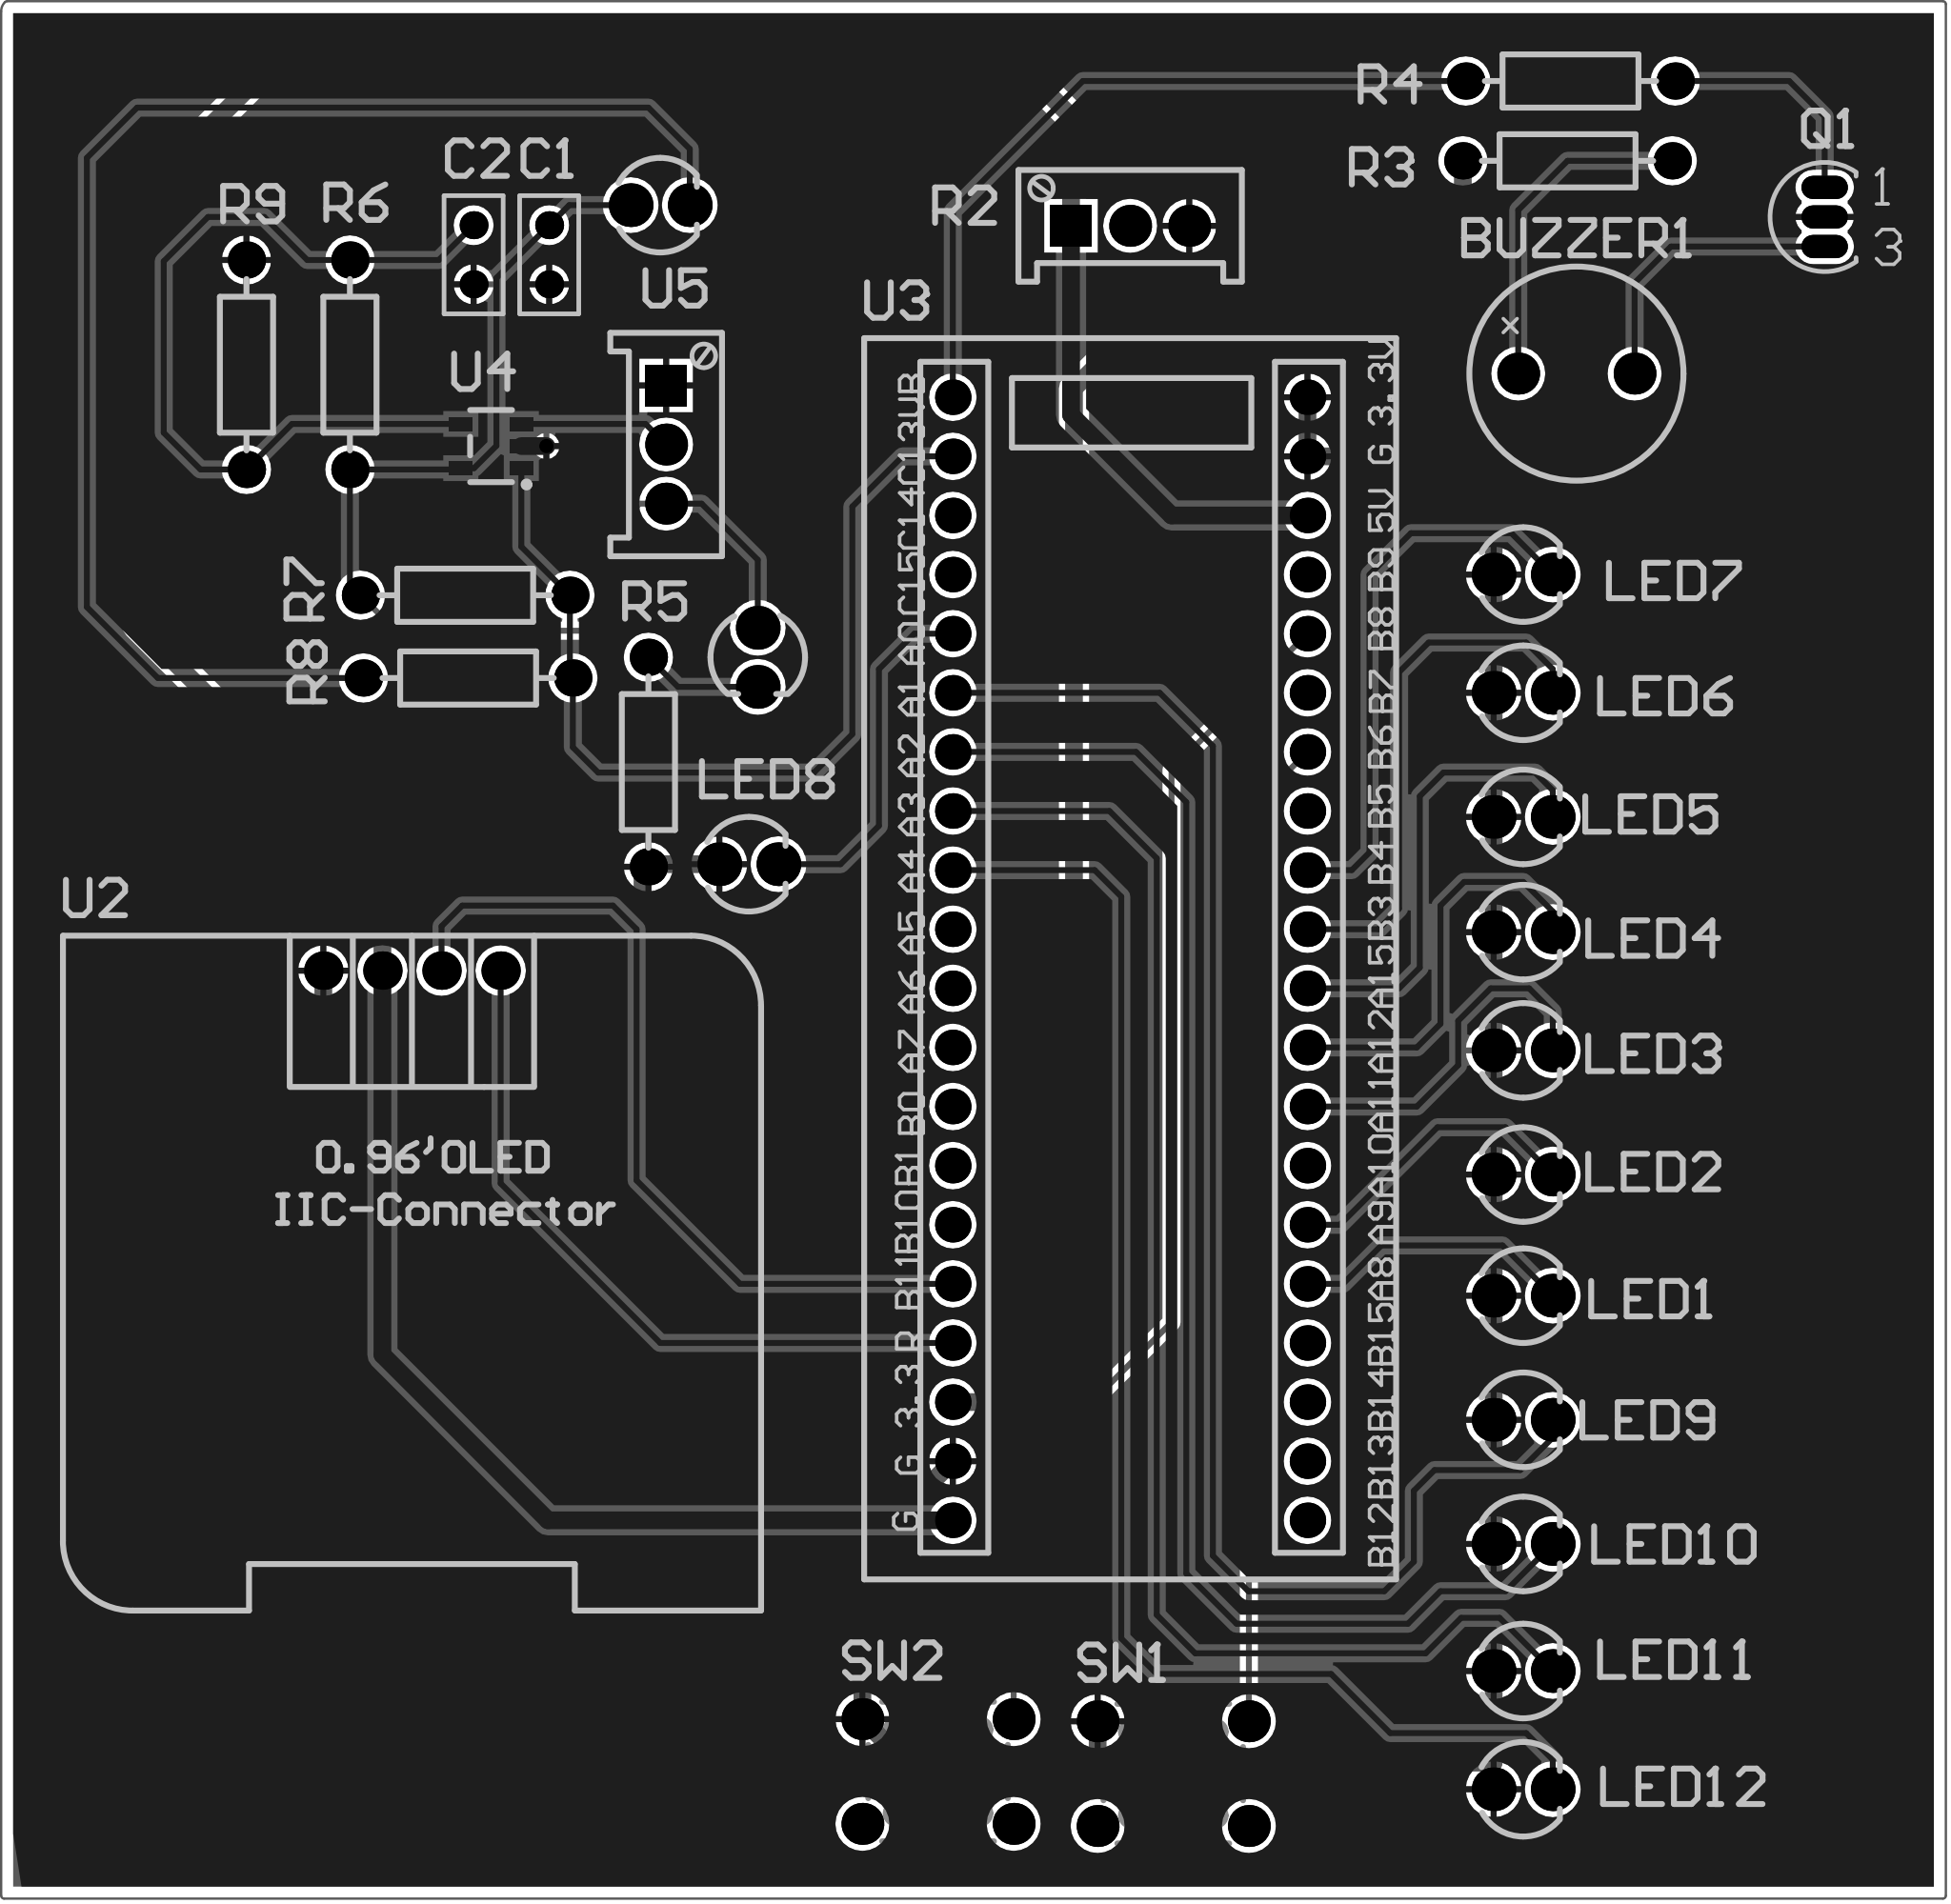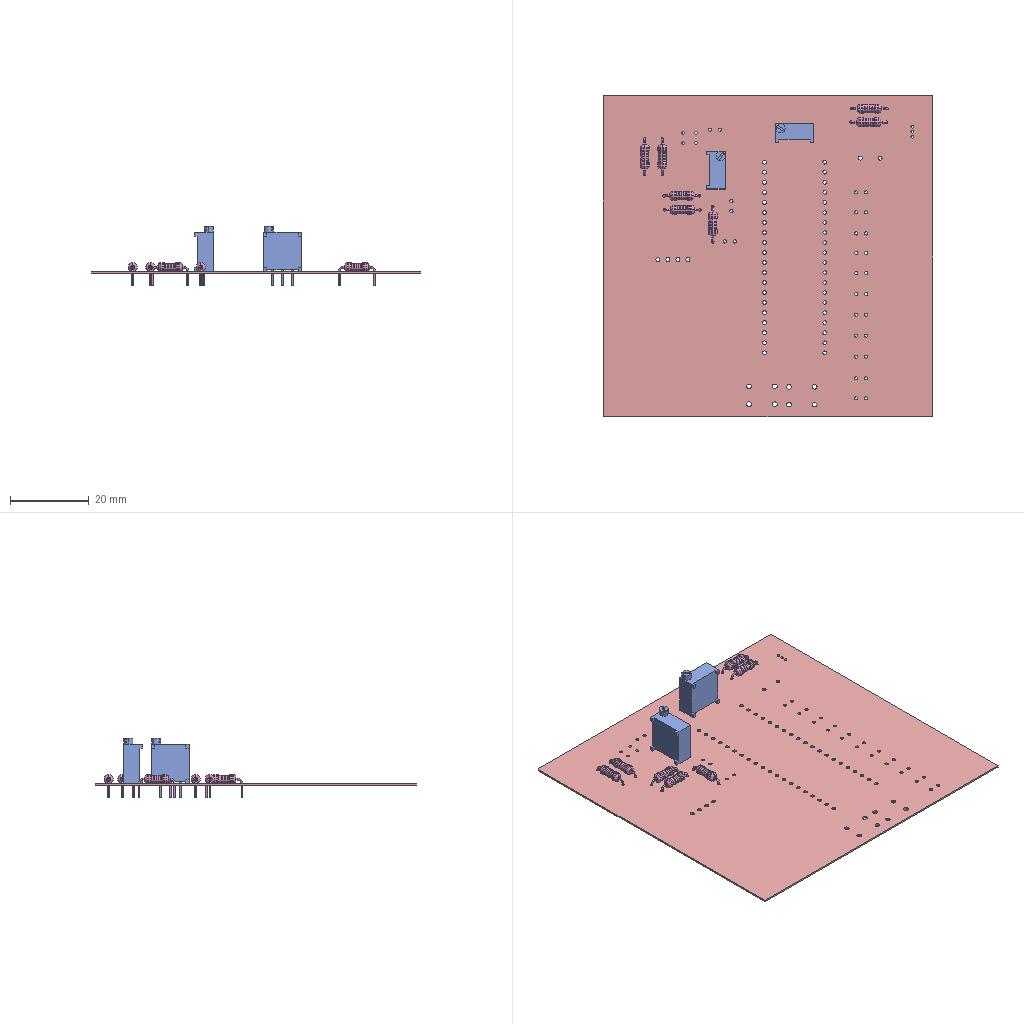Circuit board layout | Altium Designer | box 83.6 x 81.5 x 15 mm
Layer stack:
# Altium Designer layer stack of  (unit mm; dielectric type: 0 none, 1 core, 2 prepreg, 3 surface material)
index,name,kind,layer,copper_thickness_mm,dielectric_type,dielectric_thickness_mm,dielectric_material,dielectric_constant
0,Top Paste,other,,,,,,
1,Top Overlay,other,,,,,,
2,Top Solder,dielectric,,,3,0.0102,Solder Resist,3.5
3,Top Layer,copper,Top Layer,0.0356,,,,
4,Dielectric 1,dielectric,,,0,0.32,FR-4,4.8
5,Bottom Layer,copper,Bottom Layer,0.0356,,,,
6,Bottom Solder,dielectric,,,3,0.0102,Solder Resist,3.5
7,Bottom Overlay,other,,,,,,
8,Bottom Paste,other,,,,,,
# drill layer pairs: low layer,high layer
drill_pair,Top Layer,Bottom Layer
Part placement:
Designator,Comment,Layer,Footprint,Center-X(mm),Center-Y(mm),Rotation
电源指示,KT-0805G,TopLayer,LED3MM,98.933,87.503,270
开关指示,KT-0805G,TopLayer,LED3MM,94.742,106.934,360
U5,res2k3*3*1MM,TopLayer,3296W,94.996,96.647,270
U4,TLV3201AIDBVR,TopLayer,SOT-23-5_L3.0-W1.7-P0.95-LS2.8-BR,87.473,96.581,0
U3,LCKFB-DKX-STM32F103C8T6,TopLayer,STM32核心板,114.935,74.549,0
U2,HS96L03W2C03,TopLayer,0.96OLED_4P,84.074,74.04,0
SW2,TS-1101-C-W,TopLayer,四脚轻触开关,106.68,39.624,0
SW1,TS-1101-C-W,TopLayer,四脚轻触开关,116.788,39.533,0
R9,GL5506(4-7K),TopLayer,RS_1/4W,76.962,100.076,90
R8,1000Ω,TopLayer,RS_1/4W,86.487,86.614,180
R7,10000,TopLayer,RS_1/4W,86.36,90.17,180
R6,10000,TopLayer,RS_1/4W,81.407,100.076,270
R5,1000Ω,TopLayer,RS_1/4W,94.234,83.003,90
R4,1kΩ,TopLayer,RS_1/4W,133.858,112.268,360
R3,100,TopLayer,RS_1/4W,133.731,108.839,180
R2,500kΩ,TopLayer,3296W,114.935,106.045,360
Q1,SS8050,TopLayer,TO-92,144.78,106.426,360
LED12,LTST-C190KSKT,TopLayer,LED3MM,131.826,38.862,360
LED11,LTST-C190KSKT,TopLayer,LED3MM,131.826,43.942,360
LED10,LTST-C190KSKT,TopLayer,LED3MM,131.826,49.403,360
LED9,LTST-C190KSKT,TopLayer,LED3MM,131.826,54.737,0
LED8,LTST-C190KSKT,TopLayer,LED3MM,98.552,78.613,0
LED7,LTST-C190KSKT,TopLayer,LED3MM,131.826,91.059,0
LED6,LTST-C190KSKT,TopLayer,LED3MM,131.826,85.979,0
LED5,LTST-C190KSKT,TopLayer,LED3MM,131.826,80.645,0
LED4,LTST-C190KSKT,TopLayer,LED3MM,131.826,75.692,0
LED3,LTST-C190KSKT,TopLayer,LED3MM,131.826,70.612,0
LED2,LTST-C190KSKT,TopLayer,LED3MM,131.826,65.278,0
LED1,LTST-C190KSKT,TopLayer,LED3MM,131.826,60.071,0
C2,100nF,TopLayer,RAD-0.1,86.722,104.802,90
C1,104,TopLayer,RAD-0.1,89.97,104.802,90
BUZZER1,2.4kHz,TopLayer,BUZZER,134.112,99.695,360
Pad and via stacks:
# Altium Designer via and pad stacks of  (unit mm). Each distinct definition once, with the count of objects using it.
# via: kind,start_layer,end_layer,hole_mm,diameter_mm,mode(0 simple;1 top-mid-bottom;2 full stack),diameter_per_layer,count,example_net
# pad: kind,layer,hole_mm,hole_type(0 round;1 square;2 slot),plating,top_size,top_shape(1 round;2 rect;3 octagon;9 rounded rect),mid_size,bottom_size,mode,footprint,size_per_layer,count,example
pad,Multi-Layer,0.8128,2,plated,1.88x1.88,1,1.88x1.88,1.88x1.88,0,LED3MM,,28,LED2.1
pad,Multi-Layer,1,2,plated,1.65x1.65,1,1.65x1.65,1.65x1.65,0,0.96OLED_4P,,4,U2.4
pad,Multi-Layer,0.9144,2,plated,1.524x1.524,1,1.524x1.524,1.524x1.524,0,STM32\u00BA\u00CB\u00D0\u00C4\u00B0\u00E5,,40,U3.1
pad,Multi-Layer,0.7,0,plated,1.8x1.8,1,1.8x1.8,1.8x1.8,0,3296W,,4,R2.3
pad,Multi-Layer,0.7,0,plated,1.8x1.8,2,1.8x1.8,1.8x1.8,0,3296W,,2,R2.1
pad,Multi-Layer,1.2,0,plated,1.8x1.8,1,1.8x1.8,1.8x1.8,0,\u00CB\u00C4\u00BD\u00C5\u00C7\u00E1\u00B4\u00A5\u00BF\u00AA\u00B9\u00D8,,8,SW1.4
pad,Multi-Layer,0.6,0,plated,1.6x1.6,1,1.6x1.6,1.6x1.6,0,RS 1/4W,,14,R7.2
pad,Multi-Layer,0.7,0,plated,1.2x1.2,1,1.2x1.2,1.2x1.2,0,RAD-0.1,,4,C1.1
pad,Multi-Layer,1,0,plated,1.8x1.8,1,1.8x1.8,1.8x1.8,0,BUZZER,,2,BUZZER1.1
pad,Multi-Layer,0.7,0,plated,2x1,1,2x1,2x1,0,TO-92,,3,Q1.3
pad,Top Layer,0,0,plated,1x0.6,2,1x0.6,1x0.6,0,SOT-23-5_L3.0-W1.7-P0.95-LS2.8-BR,,5,U4.5
via,Top Layer,Bottom Layer,0.3048,0.6096,0,,1,GND
Copper pours:
name,layer,net,type(0 solid;1 hatched;2 none)
D,Top Layer,GND,0
D,Bottom Layer,GND,0
Design rules, without the lines most boards share:
# Altium Designer design rules of  (exported by Altium Designer, unit mm)
# columns: name | kind | enabled | priority | scope1 | scope2 | descriptor | typed fields (field=value)
SilkToSilkClearance | 55 | enabled | 1 | All | All | Silk to Silk (Clearance=0mil) (All),(All) |
SilkToSolderMaskClearance | 54 | enabled | 1 | IsPad | All | Silk To Solder Mask (Clearance=0mil) (IsPad),(All) |
MinimumSolderMaskSliver | 53 | enabled | 1 | All | All | Minimum Solder Mask Sliver (Gap=0mil) (All),(All) |
HoleToHoleClearance | 52 | enabled | 1 | All | All | Hole To Hole Clearance (Gap=10mil) (All),(All) | gap=0.254
DiffPairsRouting | 51 | enabled | 1 | All | All | Differential Pairs Uncoupled Length using the Gap Constraints (Min=10mil) (Max=10mil) (Prefered=10mil)  and Width Constraints (Min=15mil) (Max=15mil) (Prefered=15mil) (All) |
SolderMaskExpansion | 13 | enabled | 1 | All | All | Solder Mask Expansion (Expansion =4mil) (All) | expansion=0.1016
PasteMaskExpansion | 14 | enabled | 1 | All | All | Paste Mask Expansion (Expansion =0mil) (All) | expansion=0
RoutingVias | 11 | enabled | 1 | All | All | Routing Via (MinHoleWidth=28mil) (MaxHoleWidth=28mil) (PreferredHoleWidth=28mil) (MinWidth=50mil) (MaxWidth=50mil) (PreferedWidth=50mil) (All) | via_min_hole=0.7112 via_max_hole=0.7112 via_preferred_diameter=1.27 via_preferred_hole=0.7112
Width | 2 | enabled | 1 | All | All | Width Constraint (Min=10mil) (Max=30mil) (Preferred=10mil) (All) |
PolygonConnect | 20 | enabled | 1 | All | All | Polygon Connect Rule(Relief Connect )(Conductor Width=10mil) (Relief Angle=90 Angle) (Entries=4) (Air Gap Width=10mil) (All),(All) | connect_style(0=relief,1=direct,2=none)=0 relief_conductor_width=0.254 relief_entries=4
PlaneConnect | 6 | enabled | 1 | All | All | Power Plane Connect Rule(Relief Connect )(Expansion=20mil) (Conductor Width=10mil) (Air Gap=10mil) (Entries=4) (All) | relief_conductor_width=0.254 relief_entries=4 relief_expansion=0.508
Clearance | 0 | enabled | 1 | All | All | Clearance Constraint (Gap=10mil) (All),(All) | gap=0.254